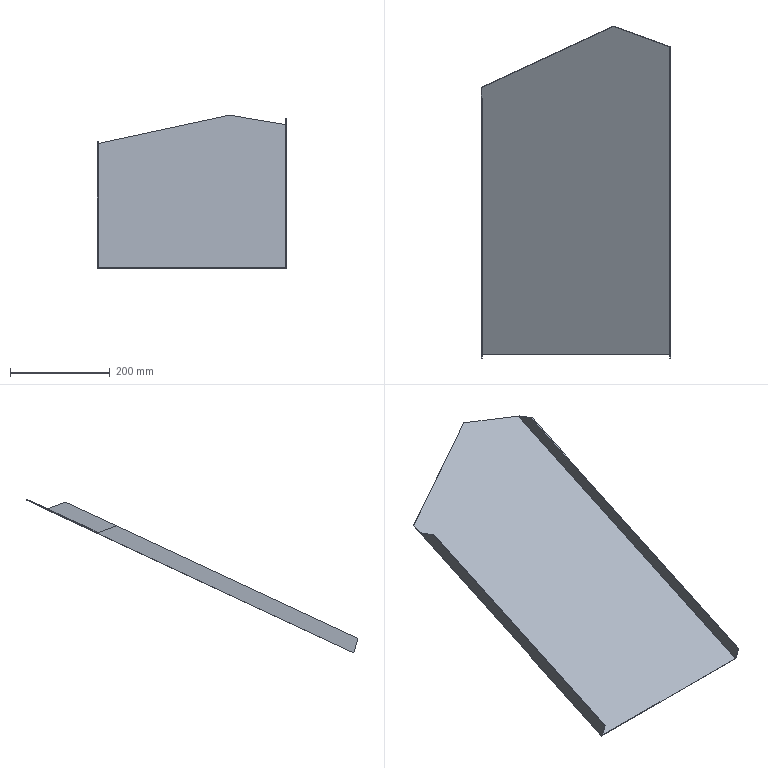Part | NX | features solid 2 | 1 solid | 13 faces | box 381.04 x 666.412 x 308.889 mm | volume 580157 mm3 | plane 12 | spline 1
STEP:
#1=CARTESIAN_POINT('',(-25.568,-610.19,-525.115));
#2=VERTEX_POINT('',#1);
#3=CARTESIAN_POINT('',(-402.608,-610.19,-525.115));
#4=VERTEX_POINT('',#3);
#5=CARTESIAN_POINT('',(-138.534,-610.19,-525.115));
#6=DIRECTION('',(-1.,0.,0.));
#7=VECTOR('',#6,1000.);
#8=LINE('',#5,#7);
#9=EDGE_CURVE('',#2,#4,#8,.T.);
#10=ORIENTED_EDGE('',*,*,#9,.F.);
#11=CARTESIAN_POINT('',(-25.568,6.211,-237.682));
#12=VERTEX_POINT('',#11);
#13=CARTESIAN_POINT('',(-25.568,48.018,-218.187));
#14=DIRECTION('',(0.,-0.9063,-0.4226));
#15=VECTOR('',#14,1000.);
#16=LINE('',#13,#15);
#17=EDGE_CURVE('',#12,#2,#16,.T.);
#18=ORIENTED_EDGE('',*,*,#17,.F.);
#19=CARTESIAN_POINT('',(-23.568,6.211,-237.682));
#20=VERTEX_POINT('',#19);
#21=CARTESIAN_POINT('',(-23.568,6.211,-237.682));
#22=DIRECTION('',(1.,0.,0.));
#23=VECTOR('',#22,1000.);
#24=LINE('',#21,#23);
#25=EDGE_CURVE('',#12,#20,#24,.T.);
#26=ORIENTED_EDGE('',*,*,#25,.T.);
#27=CARTESIAN_POINT('',(-138.534,48.018,-218.187));
#28=VERTEX_POINT('',#27);
#29=CARTESIAN_POINT('',(-23.568,6.211,-237.682));
#30=CARTESIAN_POINT('',(-27.533,7.645,-237.014));
#31=CARTESIAN_POINT('',(-35.875,10.665,-235.605));
#32=CARTESIAN_POINT('',(-47.336,14.823,-233.666));
#33=CARTESIAN_POINT('',(-57.125,18.379,-232.008));
#34=CARTESIAN_POINT('',(-63.503,20.697,-230.928));
#35=CARTESIAN_POINT('',(-68.758,22.608,-230.036));
#36=CARTESIAN_POINT('',(-72.78,24.071,-229.354));
#37=CARTESIAN_POINT('',(-76.188,25.311,-228.776));
#38=CARTESIAN_POINT('',(-78.624,26.198,-228.362));
#39=CARTESIAN_POINT('',(-80.,26.699,-228.129));
#40=CARTESIAN_POINT('',(-81.108,27.102,-227.941));
#41=CARTESIAN_POINT('',(-81.95,27.409,-227.798));
#42=CARTESIAN_POINT('',(-83.166,27.851,-227.591));
#43=CARTESIAN_POINT('',(-85.25,28.61,-227.237));
#44=CARTESIAN_POINT('',(-88.25,29.702,-226.728));
#45=CARTESIAN_POINT('',(-91.84,31.009,-226.119));
#46=CARTESIAN_POINT('',(-96.63,32.753,-225.305));
#47=CARTESIAN_POINT('',(-102.616,34.933,-224.289));
#48=CARTESIAN_POINT('',(-112.194,38.422,-222.662));
#49=CARTESIAN_POINT('',(-124.167,42.783,-220.628));
#50=CARTESIAN_POINT('',(-133.745,46.273,-219.001));
#51=CARTESIAN_POINT('',(-138.534,48.018,-218.187));
#52=B_SPLINE_CURVE_WITH_KNOTS('',3,(#29,#30,#31,#32,#33,#34,#35,#36,#37,#38,#39,#40,#41,#42,#43,#44,#45,#46,#47,#48,#49,#50,#51),.UNSPECIFIED.,.F.,.F.,(4,1,1,1,1,1,1,1,1,1,1,1,1,1,1,1,1,1,1,1,4),(0.,0.125,0.25,0.3125,0.375,0.4062,0.4375,0.4688,0.4844,0.4922,0.5,0.5078,0.5156,0.5312,0.5625,0.5938,0.625,0.6875,0.75,0.875,1.),.UNSPECIFIED.);
#53=EDGE_CURVE('',#20,#28,#52,.T.);
#54=ORIENTED_EDGE('',*,*,#53,.T.);
#55=CARTESIAN_POINT('',(-404.608,-75.034,-275.567));
#56=VERTEX_POINT('',#55);
#57=CARTESIAN_POINT('',(-138.534,48.018,-218.187));
#58=DIRECTION('',(0.8907,0.4119,0.1921));
#59=VECTOR('',#58,1000.);
#60=LINE('',#57,#59);
#61=EDGE_CURVE('',#28,#56,#60,.F.);
#62=ORIENTED_EDGE('',*,*,#61,.T.);
#63=CARTESIAN_POINT('',(-404.608,-95.845,-285.272));
#64=VERTEX_POINT('',#63);
#65=CARTESIAN_POINT('',(-404.608,48.018,-218.187));
#66=DIRECTION('',(0.,-0.9063,-0.4226));
#67=VECTOR('',#66,1000.);
#68=LINE('',#65,#67);
#69=EDGE_CURVE('',#56,#64,#68,.T.);
#70=ORIENTED_EDGE('',*,*,#69,.T.);
#71=CARTESIAN_POINT('',(-402.608,-95.845,-285.272));
#72=VERTEX_POINT('',#71);
#73=CARTESIAN_POINT('',(-449.608,-95.845,-285.272));
#74=DIRECTION('',(-1.,0.,0.));
#75=VECTOR('',#74,1000.);
#76=LINE('',#73,#75);
#77=EDGE_CURVE('',#64,#72,#76,.F.);
#78=ORIENTED_EDGE('',*,*,#77,.T.);
#79=CARTESIAN_POINT('',(-402.608,48.018,-218.187));
#80=DIRECTION('',(0.,-0.9063,-0.4226));
#81=VECTOR('',#80,1000.);
#82=LINE('',#79,#81);
#83=EDGE_CURVE('',#72,#4,#82,.T.);
#84=ORIENTED_EDGE('',*,*,#83,.T.);
#85=EDGE_LOOP('',(#10,#18,#26,#54,#62,#70,#78,#84));
#86=FACE_BOUND('',#85,.T.);
#87=CARTESIAN_POINT('',(-138.534,48.018,-218.187));
#88=DIRECTION('',(0.,-0.4226,0.9063));
#89=DIRECTION('',(1.,0.,0.));
#90=AXIS2_PLACEMENT_3D('',#87,#88,#89);
#91=PLANE('',#90);
#92=ADVANCED_FACE('',(#86),#91,.T.);
#93=CARTESIAN_POINT('',(-23.568,-609.664,-527.076));
#94=VERTEX_POINT('',#93);
#95=CARTESIAN_POINT('',(-23.568,-617.549,-497.651));
#96=VERTEX_POINT('',#95);
#97=CARTESIAN_POINT('',(-23.568,-642.83,-403.3));
#98=DIRECTION('',(0.,-0.2588,0.9659));
#99=VECTOR('',#98,1000.);
#100=LINE('',#97,#99);
#101=EDGE_CURVE('',#94,#96,#100,.T.);
#102=ORIENTED_EDGE('',*,*,#101,.F.);
#103=CARTESIAN_POINT('',(-23.568,7.056,-239.495));
#104=VERTEX_POINT('',#103);
#105=CARTESIAN_POINT('',(-23.568,48.863,-220.));
#106=DIRECTION('',(0.,-0.9063,-0.4226));
#107=VECTOR('',#106,1000.);
#108=LINE('',#105,#107);
#109=EDGE_CURVE('',#104,#94,#108,.T.);
#110=ORIENTED_EDGE('',*,*,#109,.F.);
#111=CARTESIAN_POINT('',(-23.568,7.056,-239.495));
#112=CARTESIAN_POINT('',(-23.568,6.775,-238.891));
#113=CARTESIAN_POINT('',(-23.568,6.493,-238.286));
#114=CARTESIAN_POINT('',(-23.568,6.211,-237.682));
#115=B_SPLINE_CURVE_WITH_KNOTS('',3,(#111,#112,#113,#114),.UNSPECIFIED.,.F.,.F.,(4,4),(0.,1.),.UNSPECIFIED.);
#116=EDGE_CURVE('',#20,#104,#115,.F.);
#117=ORIENTED_EDGE('',*,*,#116,.F.);
#118=CARTESIAN_POINT('',(-23.568,-30.999,-224.139));
#119=VERTEX_POINT('',#118);
#120=CARTESIAN_POINT('',(-23.568,-30.999,-224.139));
#121=DIRECTION('',(0.,0.9397,-0.342));
#122=VECTOR('',#121,1000.);
#123=LINE('',#120,#122);
#124=EDGE_CURVE('',#20,#119,#123,.F.);
#125=ORIENTED_EDGE('',*,*,#124,.T.);
#126=CARTESIAN_POINT('',(-23.568,-5.622,-212.306));
#127=DIRECTION('',(0.,-0.9063,-0.4226));
#128=VECTOR('',#127,1000.);
#129=LINE('',#126,#128);
#130=EDGE_CURVE('',#119,#96,#129,.T.);
#131=ORIENTED_EDGE('',*,*,#130,.T.);
#132=EDGE_LOOP('',(#102,#110,#117,#125,#131));
#133=FACE_BOUND('',#132,.T.);
#134=CARTESIAN_POINT('',(-23.568,48.018,-218.187));
#135=DIRECTION('',(1.,0.,0.));
#136=DIRECTION('',(0.,1.,0.));
#137=AXIS2_PLACEMENT_3D('',#134,#135,#136);
#138=PLANE('',#137);
#139=ADVANCED_FACE('',(#133),#138,.T.);
#140=CARTESIAN_POINT('',(-138.534,48.863,-220.));
#141=VERTEX_POINT('',#140);
#142=CARTESIAN_POINT('',(-23.568,7.056,-239.495));
#143=CARTESIAN_POINT('',(-27.533,8.49,-238.826));
#144=CARTESIAN_POINT('',(-35.875,11.511,-237.418));
#145=CARTESIAN_POINT('',(-47.336,15.668,-235.479));
#146=CARTESIAN_POINT('',(-57.125,19.224,-233.821));
#147=CARTESIAN_POINT('',(-63.503,21.542,-232.74));
#148=CARTESIAN_POINT('',(-68.758,23.453,-231.849));
#149=CARTESIAN_POINT('',(-72.78,24.916,-231.167));
#150=CARTESIAN_POINT('',(-76.188,26.156,-230.588));
#151=CARTESIAN_POINT('',(-78.624,27.043,-230.175));
#152=CARTESIAN_POINT('',(-80.,27.544,-229.941));
#153=CARTESIAN_POINT('',(-81.108,27.947,-229.753));
#154=CARTESIAN_POINT('',(-81.95,28.254,-229.61));
#155=CARTESIAN_POINT('',(-83.166,28.696,-229.404));
#156=CARTESIAN_POINT('',(-85.25,29.455,-229.05));
#157=CARTESIAN_POINT('',(-88.25,30.547,-228.541));
#158=CARTESIAN_POINT('',(-91.84,31.854,-227.931));
#159=CARTESIAN_POINT('',(-96.63,33.599,-227.118));
#160=CARTESIAN_POINT('',(-102.616,35.779,-226.101));
#161=CARTESIAN_POINT('',(-112.194,39.267,-224.475));
#162=CARTESIAN_POINT('',(-124.167,43.628,-222.441));
#163=CARTESIAN_POINT('',(-133.745,47.118,-220.814));
#164=CARTESIAN_POINT('',(-138.534,48.863,-220.));
#165=B_SPLINE_CURVE_WITH_KNOTS('',3,(#142,#143,#144,#145,#146,#147,#148,#149,#150,#151,#152,#153,#154,#155,#156,#157,#158,#159,#160,#161,#162,#163,#164),.UNSPECIFIED.,.F.,.F.,(4,1,1,1,1,1,1,1,1,1,1,1,1,1,1,1,1,1,1,1,4),(0.,0.125,0.25,0.3125,0.375,0.4062,0.4375,0.4688,0.4844,0.4922,0.5,0.5078,0.5156,0.5312,0.5625,0.5938,0.625,0.6875,0.75,0.875,1.),.UNSPECIFIED.);
#166=EDGE_CURVE('',#104,#141,#165,.T.);
#167=ORIENTED_EDGE('',*,*,#166,.T.);
#168=CARTESIAN_POINT('',(-138.534,48.018,-218.187));
#169=CARTESIAN_POINT('',(-138.534,48.3,-218.792));
#170=CARTESIAN_POINT('',(-138.534,48.581,-219.396));
#171=CARTESIAN_POINT('',(-138.534,48.863,-220.));
#172=B_SPLINE_CURVE_WITH_KNOTS('',3,(#168,#169,#170,#171),.UNSPECIFIED.,.F.,.F.,(4,4),(0.,1.),.UNSPECIFIED.);
#173=EDGE_CURVE('',#28,#141,#172,.T.);
#174=ORIENTED_EDGE('',*,*,#173,.F.);
#175=ORIENTED_EDGE('',*,*,#53,.F.);
#176=ORIENTED_EDGE('',*,*,#116,.T.);
#177=EDGE_LOOP('',(#167,#174,#175,#176));
#178=FACE_BOUND('',#177,.T.);
#179=CARTESIAN_POINT('',(-23.568,6.211,-237.682));
#180=CARTESIAN_POINT('',(-23.568,7.056,-239.495));
#181=CARTESIAN_POINT('',(-27.533,7.645,-237.014));
#182=CARTESIAN_POINT('',(-27.533,8.49,-238.826));
#183=CARTESIAN_POINT('',(-35.875,10.665,-235.605));
#184=CARTESIAN_POINT('',(-35.875,11.511,-237.418));
#185=CARTESIAN_POINT('',(-47.336,14.823,-233.666));
#186=CARTESIAN_POINT('',(-47.336,15.668,-235.479));
#187=CARTESIAN_POINT('',(-57.125,18.379,-232.008));
#188=CARTESIAN_POINT('',(-57.125,19.224,-233.821));
#189=CARTESIAN_POINT('',(-63.503,20.697,-230.928));
#190=CARTESIAN_POINT('',(-63.503,21.542,-232.74));
#191=CARTESIAN_POINT('',(-68.758,22.608,-230.036));
#192=CARTESIAN_POINT('',(-68.758,23.453,-231.849));
#193=CARTESIAN_POINT('',(-72.78,24.071,-229.354));
#194=CARTESIAN_POINT('',(-72.78,24.916,-231.167));
#195=CARTESIAN_POINT('',(-76.188,25.311,-228.776));
#196=CARTESIAN_POINT('',(-76.188,26.156,-230.588));
#197=CARTESIAN_POINT('',(-78.624,26.198,-228.362));
#198=CARTESIAN_POINT('',(-78.624,27.043,-230.175));
#199=CARTESIAN_POINT('',(-80.,26.699,-228.129));
#200=CARTESIAN_POINT('',(-80.,27.544,-229.941));
#201=CARTESIAN_POINT('',(-81.108,27.102,-227.941));
#202=CARTESIAN_POINT('',(-81.108,27.947,-229.753));
#203=CARTESIAN_POINT('',(-81.95,27.409,-227.798));
#204=CARTESIAN_POINT('',(-81.95,28.254,-229.61));
#205=CARTESIAN_POINT('',(-83.166,27.851,-227.591));
#206=CARTESIAN_POINT('',(-83.166,28.696,-229.404));
#207=CARTESIAN_POINT('',(-85.25,28.61,-227.237));
#208=CARTESIAN_POINT('',(-85.25,29.455,-229.05));
#209=CARTESIAN_POINT('',(-88.25,29.702,-226.728));
#210=CARTESIAN_POINT('',(-88.25,30.547,-228.541));
#211=CARTESIAN_POINT('',(-91.84,31.009,-226.119));
#212=CARTESIAN_POINT('',(-91.84,31.854,-227.931));
#213=CARTESIAN_POINT('',(-96.63,32.753,-225.305));
#214=CARTESIAN_POINT('',(-96.63,33.599,-227.118));
#215=CARTESIAN_POINT('',(-102.616,34.933,-224.289));
#216=CARTESIAN_POINT('',(-102.616,35.779,-226.101));
#217=CARTESIAN_POINT('',(-112.194,38.422,-222.662));
#218=CARTESIAN_POINT('',(-112.194,39.267,-224.475));
#219=CARTESIAN_POINT('',(-124.167,42.783,-220.628));
#220=CARTESIAN_POINT('',(-124.167,43.628,-222.441));
#221=CARTESIAN_POINT('',(-133.745,46.273,-219.001));
#222=CARTESIAN_POINT('',(-133.745,47.118,-220.814));
#223=CARTESIAN_POINT('',(-138.534,48.018,-218.187));
#224=CARTESIAN_POINT('',(-138.534,48.863,-220.));
#225=B_SPLINE_SURFACE_WITH_KNOTS('',3,1,((#179,#180),(#181,#182),(#183,#184),(#185,#186),(#187,#188),(#189,#190),(#191,#192),(#193,#194),(#195,#196),(#197,#198),(#199,#200),(#201,#202),(#203,#204),(#205,#206),(#207,#208),(#209,#210),(#211,#212),(#213,#214),(#215,#216),(#217,#218),(#219,#220),(#221,#222),(#223,#224)),.SURF_OF_LINEAR_EXTRUSION.,.F.,.F.,.F.,(4,1,1,1,1,1,1,1,1,1,1,1,1,1,1,1,1,1,1,1,4),(2,2),(0.,0.125,0.25,0.3125,0.375,0.4062,0.4375,0.4688,0.4844,0.4922,0.5,0.5078,0.5156,0.5312,0.5625,0.5938,0.625,0.6875,0.75,0.875,1.),(0.,1.),.UNSPECIFIED.);
#226=ADVANCED_FACE('',(#178),#225,.F.);
#227=CARTESIAN_POINT('',(-404.608,-74.189,-277.38));
#228=VERTEX_POINT('',#227);
#229=CARTESIAN_POINT('',(-138.534,48.863,-220.));
#230=DIRECTION('',(0.8907,0.4119,0.1921));
#231=VECTOR('',#230,1000.);
#232=LINE('',#229,#231);
#233=EDGE_CURVE('',#141,#228,#232,.F.);
#234=ORIENTED_EDGE('',*,*,#233,.T.);
#235=CARTESIAN_POINT('',(-404.608,-75.034,-275.567));
#236=DIRECTION('',(0.,0.4226,-0.9063));
#237=VECTOR('',#236,1000.);
#238=LINE('',#235,#237);
#239=EDGE_CURVE('',#56,#228,#238,.T.);
#240=ORIENTED_EDGE('',*,*,#239,.F.);
#241=ORIENTED_EDGE('',*,*,#61,.F.);
#242=ORIENTED_EDGE('',*,*,#173,.T.);
#243=EDGE_LOOP('',(#234,#240,#241,#242));
#244=FACE_BOUND('',#243,.T.);
#245=CARTESIAN_POINT('',(-138.534,48.018,-218.187));
#246=DIRECTION('',(0.4545,-0.8073,-0.3764));
#247=DIRECTION('',(0.8714,0.4906,0.));
#248=AXIS2_PLACEMENT_3D('',#245,#246,#247);
#249=PLANE('',#248);
#250=ADVANCED_FACE('',(#244),#249,.F.);
#251=CARTESIAN_POINT('',(-404.608,-609.664,-527.076));
#252=VERTEX_POINT('',#251);
#253=CARTESIAN_POINT('',(-404.608,48.863,-220.));
#254=DIRECTION('',(0.,-0.9063,-0.4226));
#255=VECTOR('',#254,1000.);
#256=LINE('',#253,#255);
#257=EDGE_CURVE('',#228,#252,#256,.T.);
#258=ORIENTED_EDGE('',*,*,#257,.T.);
#259=CARTESIAN_POINT('',(-404.608,-617.549,-497.651));
#260=VERTEX_POINT('',#259);
#261=CARTESIAN_POINT('',(-404.608,-642.83,-403.3));
#262=DIRECTION('',(0.,-0.2588,0.9659));
#263=VECTOR('',#262,1000.);
#264=LINE('',#261,#263);
#265=EDGE_CURVE('',#252,#260,#264,.T.);
#266=ORIENTED_EDGE('',*,*,#265,.T.);
#267=CARTESIAN_POINT('',(-404.608,-133.055,-271.729));
#268=VERTEX_POINT('',#267);
#269=CARTESIAN_POINT('',(-404.608,36.185,-192.811));
#270=DIRECTION('',(0.,0.9063,0.4226));
#271=VECTOR('',#270,1000.);
#272=LINE('',#269,#271);
#273=EDGE_CURVE('',#268,#260,#272,.F.);
#274=ORIENTED_EDGE('',*,*,#273,.F.);
#275=CARTESIAN_POINT('',(-404.608,-95.845,-285.272));
#276=DIRECTION('',(0.,-0.9397,0.342));
#277=VECTOR('',#276,1000.);
#278=LINE('',#275,#277);
#279=EDGE_CURVE('',#268,#64,#278,.F.);
#280=ORIENTED_EDGE('',*,*,#279,.T.);
#281=ORIENTED_EDGE('',*,*,#69,.F.);
#282=ORIENTED_EDGE('',*,*,#239,.T.);
#283=EDGE_LOOP('',(#258,#266,#274,#280,#281,#282));
#284=FACE_BOUND('',#283,.T.);
#285=CARTESIAN_POINT('',(-404.608,48.018,-218.187));
#286=DIRECTION('',(1.,0.,0.));
#287=DIRECTION('',(0.,1.,0.));
#288=AXIS2_PLACEMENT_3D('',#285,#286,#287);
#289=PLANE('',#288);
#290=ADVANCED_FACE('',(#284),#289,.F.);
#291=ORIENTED_EDGE('',*,*,#109,.T.);
#292=CARTESIAN_POINT('',(-138.534,-609.664,-527.076));
#293=DIRECTION('',(-1.,0.,0.));
#294=VECTOR('',#293,1000.);
#295=LINE('',#292,#294);
#296=EDGE_CURVE('',#94,#252,#295,.T.);
#297=ORIENTED_EDGE('',*,*,#296,.T.);
#298=ORIENTED_EDGE('',*,*,#257,.F.);
#299=ORIENTED_EDGE('',*,*,#233,.F.);
#300=ORIENTED_EDGE('',*,*,#166,.F.);
#301=EDGE_LOOP('',(#291,#297,#298,#299,#300));
#302=FACE_BOUND('',#301,.T.);
#303=CARTESIAN_POINT('',(-138.534,48.863,-220.));
#304=DIRECTION('',(0.,-0.4226,0.9063));
#305=DIRECTION('',(1.,0.,0.));
#306=AXIS2_PLACEMENT_3D('',#303,#304,#305);
#307=PLANE('',#306);
#308=ADVANCED_FACE('',(#302),#307,.F.);
#309=CARTESIAN_POINT('',(-402.608,-617.549,-497.651));
#310=VERTEX_POINT('',#309);
#311=CARTESIAN_POINT('',(-449.608,-617.549,-497.651));
#312=DIRECTION('',(1.,0.,0.));
#313=VECTOR('',#312,1000.);
#314=LINE('',#311,#313);
#315=EDGE_CURVE('',#310,#260,#314,.F.);
#316=ORIENTED_EDGE('',*,*,#315,.F.);
#317=CARTESIAN_POINT('',(-402.608,-133.055,-271.729));
#318=VERTEX_POINT('',#317);
#319=CARTESIAN_POINT('',(-402.608,-107.679,-259.895));
#320=DIRECTION('',(0.,0.9063,0.4226));
#321=VECTOR('',#320,1000.);
#322=LINE('',#319,#321);
#323=EDGE_CURVE('',#318,#310,#322,.F.);
#324=ORIENTED_EDGE('',*,*,#323,.F.);
#325=CARTESIAN_POINT('',(-449.608,-133.055,-271.729));
#326=DIRECTION('',(1.,0.,0.));
#327=VECTOR('',#326,1000.);
#328=LINE('',#325,#327);
#329=EDGE_CURVE('',#318,#268,#328,.F.);
#330=ORIENTED_EDGE('',*,*,#329,.T.);
#331=ORIENTED_EDGE('',*,*,#273,.T.);
#332=EDGE_LOOP('',(#316,#324,#330,#331));
#333=FACE_BOUND('',#332,.T.);
#334=CARTESIAN_POINT('',(-449.608,-107.679,-259.895));
#335=DIRECTION('',(0.,0.4226,-0.9063));
#336=DIRECTION('',(0.,-0.9063,-0.4226));
#337=AXIS2_PLACEMENT_3D('',#334,#335,#336);
#338=PLANE('',#337);
#339=ADVANCED_FACE('',(#333),#338,.F.);
#340=ORIENTED_EDGE('',*,*,#323,.T.);
#341=CARTESIAN_POINT('',(-402.608,-635.186,-431.827));
#342=DIRECTION('',(0.,0.2588,-0.9659));
#343=VECTOR('',#342,1000.);
#344=LINE('',#341,#343);
#345=EDGE_CURVE('',#310,#4,#344,.T.);
#346=ORIENTED_EDGE('',*,*,#345,.T.);
#347=ORIENTED_EDGE('',*,*,#83,.F.);
#348=CARTESIAN_POINT('',(-402.608,-95.845,-285.272));
#349=DIRECTION('',(0.,0.9397,-0.342));
#350=VECTOR('',#349,1000.);
#351=LINE('',#348,#350);
#352=EDGE_CURVE('',#72,#318,#351,.F.);
#353=ORIENTED_EDGE('',*,*,#352,.T.);
#354=EDGE_LOOP('',(#340,#346,#347,#353));
#355=FACE_BOUND('',#354,.T.);
#356=CARTESIAN_POINT('',(-402.608,-95.,-287.084));
#357=DIRECTION('',(-1.,0.,0.));
#358=DIRECTION('',(0.,-1.,0.));
#359=AXIS2_PLACEMENT_3D('',#356,#357,#358);
#360=PLANE('',#359);
#361=ADVANCED_FACE('',(#355),#360,.F.);
#362=ORIENTED_EDGE('',*,*,#279,.F.);
#363=ORIENTED_EDGE('',*,*,#329,.F.);
#364=ORIENTED_EDGE('',*,*,#352,.F.);
#365=ORIENTED_EDGE('',*,*,#77,.F.);
#366=EDGE_LOOP('',(#362,#363,#364,#365));
#367=FACE_BOUND('',#366,.T.);
#368=CARTESIAN_POINT('',(-449.608,-95.845,-285.272));
#369=DIRECTION('',(0.,-0.342,-0.9397));
#370=DIRECTION('',(0.,0.9397,-0.342));
#371=AXIS2_PLACEMENT_3D('',#368,#369,#370);
#372=PLANE('',#371);
#373=ADVANCED_FACE('',(#367),#372,.F.);
#374=CARTESIAN_POINT('',(-25.568,-30.999,-224.139));
#375=VERTEX_POINT('',#374);
#376=CARTESIAN_POINT('',(-25.568,-617.549,-497.651));
#377=VERTEX_POINT('',#376);
#378=CARTESIAN_POINT('',(-25.568,-5.622,-212.306));
#379=DIRECTION('',(0.,-0.9063,-0.4226));
#380=VECTOR('',#379,1000.);
#381=LINE('',#378,#380);
#382=EDGE_CURVE('',#375,#377,#381,.T.);
#383=ORIENTED_EDGE('',*,*,#382,.T.);
#384=CARTESIAN_POINT('',(-23.568,-617.549,-497.651));
#385=DIRECTION('',(1.,0.,0.));
#386=VECTOR('',#385,1000.);
#387=LINE('',#384,#386);
#388=EDGE_CURVE('',#377,#96,#387,.T.);
#389=ORIENTED_EDGE('',*,*,#388,.T.);
#390=ORIENTED_EDGE('',*,*,#130,.F.);
#391=CARTESIAN_POINT('',(-23.568,-30.999,-224.139));
#392=DIRECTION('',(-1.,0.,0.));
#393=VECTOR('',#392,1000.);
#394=LINE('',#391,#393);
#395=EDGE_CURVE('',#119,#375,#394,.T.);
#396=ORIENTED_EDGE('',*,*,#395,.T.);
#397=EDGE_LOOP('',(#383,#389,#390,#396));
#398=FACE_BOUND('',#397,.T.);
#399=CARTESIAN_POINT('',(-23.568,-5.622,-212.306));
#400=DIRECTION('',(0.,0.4226,-0.9063));
#401=DIRECTION('',(0.,-0.9063,-0.4226));
#402=AXIS2_PLACEMENT_3D('',#399,#400,#401);
#403=PLANE('',#402);
#404=ADVANCED_FACE('',(#398),#403,.F.);
#405=CARTESIAN_POINT('',(-25.568,-640.247,-412.939));
#406=DIRECTION('',(0.,0.2588,-0.9659));
#407=VECTOR('',#406,1000.);
#408=LINE('',#405,#407);
#409=EDGE_CURVE('',#377,#2,#408,.T.);
#410=ORIENTED_EDGE('',*,*,#409,.F.);
#411=ORIENTED_EDGE('',*,*,#382,.F.);
#412=CARTESIAN_POINT('',(-25.568,7.54,-238.166));
#413=DIRECTION('',(0.,-0.9397,0.342));
#414=VECTOR('',#413,1000.);
#415=LINE('',#412,#414);
#416=EDGE_CURVE('',#375,#12,#415,.F.);
#417=ORIENTED_EDGE('',*,*,#416,.T.);
#418=ORIENTED_EDGE('',*,*,#17,.T.);
#419=EDGE_LOOP('',(#410,#411,#417,#418));
#420=FACE_BOUND('',#419,.T.);
#421=CARTESIAN_POINT('',(-25.568,7.056,-239.495));
#422=DIRECTION('',(-1.,0.,0.));
#423=DIRECTION('',(0.,-1.,0.));
#424=AXIS2_PLACEMENT_3D('',#421,#422,#423);
#425=PLANE('',#424);
#426=ADVANCED_FACE('',(#420),#425,.T.);
#427=ORIENTED_EDGE('',*,*,#124,.F.);
#428=ORIENTED_EDGE('',*,*,#25,.F.);
#429=ORIENTED_EDGE('',*,*,#416,.F.);
#430=ORIENTED_EDGE('',*,*,#395,.F.);
#431=EDGE_LOOP('',(#427,#428,#429,#430));
#432=FACE_BOUND('',#431,.T.);
#433=CARTESIAN_POINT('',(-23.568,-30.999,-224.139));
#434=DIRECTION('',(0.,-0.342,-0.9397));
#435=DIRECTION('',(0.,0.9397,-0.342));
#436=AXIS2_PLACEMENT_3D('',#433,#434,#435);
#437=PLANE('',#436);
#438=ADVANCED_FACE('',(#432),#437,.F.);
#439=ORIENTED_EDGE('',*,*,#265,.F.);
#440=ORIENTED_EDGE('',*,*,#296,.F.);
#441=ORIENTED_EDGE('',*,*,#101,.T.);
#442=ORIENTED_EDGE('',*,*,#388,.F.);
#443=ORIENTED_EDGE('',*,*,#409,.T.);
#444=ORIENTED_EDGE('',*,*,#9,.T.);
#445=ORIENTED_EDGE('',*,*,#345,.F.);
#446=ORIENTED_EDGE('',*,*,#315,.T.);
#447=EDGE_LOOP('',(#439,#440,#441,#442,#443,#444,#445,#446));
#448=FACE_BOUND('',#447,.T.);
#449=CARTESIAN_POINT('',(-414.608,-617.98,-496.043));
#450=DIRECTION('',(0.,0.9659,0.2588));
#451=DIRECTION('',(0.,-0.2588,0.9659));
#452=AXIS2_PLACEMENT_3D('',#449,#450,#451);
#453=PLANE('',#452);
#454=ADVANCED_FACE('',(#448),#453,.F.);
#455=CLOSED_SHELL('',(#92,#139,#226,#250,#290,#308,#339,#361,#373,#404,#426,#438,#454));
#456=MANIFOLD_SOLID_BREP('',#455);
#457=(LENGTH_UNIT()NAMED_UNIT(*)SI_UNIT(.MILLI.,.METRE.));
#458=UNCERTAINTY_MEASURE_WITH_UNIT(LENGTH_MEASURE(0.0508),#457,'','');
#459=(NAMED_UNIT(*)PLANE_ANGLE_UNIT()SI_UNIT($,.RADIAN.));
#460=(NAMED_UNIT(*)SI_UNIT($,.STERADIAN.)SOLID_ANGLE_UNIT());
#461=(GEOMETRIC_REPRESENTATION_CONTEXT(3)GLOBAL_UNCERTAINTY_ASSIGNED_CONTEXT((#458))GLOBAL_UNIT_ASSIGNED_CONTEXT((#457,#459,#460))REPRESENTATION_CONTEXT('',''));
#462=ADVANCED_BREP_SHAPE_REPRESENTATION('',(#456),#461);